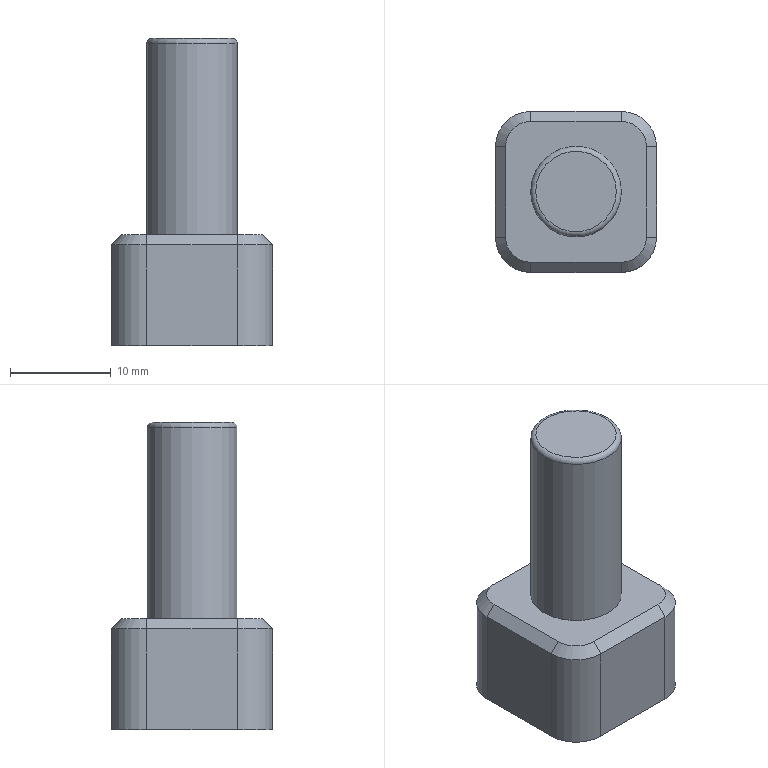NC program | NX | posted with a generic post | part box 16 x 16 x 30.5 mm
Whole program:
N10 G17 G21 G94 G90
(DYNAMIC_ROUGH , TOOL : D12-36-D12-75-3T_ROUGH)
N12 T01 M6
N14 G53
N16 G17 G0 G90 X-22.031 Y-0.836 S6500 M3
N18 G43 Z51. H1
N20 Z-31.5
N22 G94 G1 X-22.006 Z-31.656 F3000.
N24 X-21.981 Z-31.718
N26 X-21.956 Z-31.763
N28 X-21.931 Y-0.835 Z-31.8
N30 X-21.906 Z-31.831
N32 X-21.881 Z-31.857
N34 X-21.856 Y-0.834 Z-31.88
N36 X-21.831 Z-31.9
N38 X-21.806 Z-31.918
N40 X-21.781 Y-0.833 Z-31.933
N42 X-21.756 Z-31.947
N44 X-21.731 Z-31.958
N46 X-21.706 Z-31.968
N48 X-21.681 Y-0.832 Z-31.977
N50 X-21.656 Z-31.984
N52 X-21.631 Z-31.99
N54 X-21.606 Y-0.831 Z-31.994
N56 X-21.581 Z-31.997
N58 X-21.556 Z-31.999
N60 X-21.531 Y-0.83 Z-32.
N62 X-19.634 Y-0.808
N64 G3 X-18.514 Y-0.022 R1.212
N66 X-17.509 Y3.609 R109.508
N68 G2 X-12.877 Y12.031 R20.094
N70 X-4.609 Y-16.993 R-17.608
N72 X-17.194 Y-3.694 R17.471
N74 X-16.874 Y2.692 R16.424
N76 X-10.325 Y13.171 R18.361
N78 X0.613 Y-16.701 R-16.719
N80 X-15.618 Y-5.888 R16.611
N82 X-15.923 Y2.853 R15.623
N84 X-12.605 Y9.692 R17.498
N86 G1 X-12.372 Y10.081
N88 X-11.422 Y11.223
N90 G2 X4.265 Y15.209 R16.422
N92 X8.789 Y13.136 R16.46
N94 G1 X10.173 Y12.306
N96 X11.324 Y11.323
N98 G2 X15.746 Y-1.31 R16.696
N100 X13.113 Y-8.829 R16.055
N102 G1 X12.465 Y-9.948
N104 X11.561 Y-11.077
N106 G2 X6.151 Y-14.604 R15.975
N108 X-8.666 Y-13.208 R15.981
N110 G1 X-9.956 Y-12.46
N112 X-11.085 Y-11.554
N114 G2 X-15.107 Y2.306 R15.032
N116 X-14.081 Y5.563 R21.458
N118 G1 X-14.035 Y5.983
N120 X-13.695 Y7.429
N122 X-13.136 Y8.806
N124 X-12.372 Y10.081
N126 X-11.422 Y11.223
N128 X-10.308 Y12.206
N130 X-9.056 Y13.007
N132 X-7.696 Y13.605
N134 G2 X-4.061 Y14.572 R59.469
N136 X4.693 Y14.136 R17.004
N138 G1 X6.011 Y14.031
N140 X7.483 Y13.677
N142 X8.813 Y13.126
N144 X7.483 Y13.677
N146 X6.011 Y14.031
N148 G2 X1.513 Y14.441 R319.051
N150 G3 X-3.781 Y14.15 R19.844
N152 X-7.217 Y13.733 R9.939
N154 G2 X-4.48 Y14.149 R9.046
N156 G1 X4.501 Y14.15
N158 X6.011 Y14.031
N160 X7.483 Y13.677
N162 X8.882 Y13.098
N164 X10.173 Y12.306
N166 X11.324 Y11.323
N168 X12.308 Y10.171
N170 X13.099 Y8.88
N172 G2 X14.216 Y5.603 R17.673
N174 X14.691 Y-2.504 R18.171
N176 X14.133 Y-4.728 R33.317
N178 X13.099 Y-8.853 R9.647
N180 G3 X14.133 Y-4.728 R9.657
N182 X14.475 Y-0.898 R93.828
N184 X14.15 Y3.737 R22.162
N186 X14.031 Y6.008 R16.89
N188 G1 X13.678 Y7.481
N190 X14.031 Y6.008
N192 G2 X14.15 Y3.737 R16.89
N194 G1 Y-4.501
N196 X14.041 Y-5.943
N198 X13.719 Y-7.352
N200 X13.189 Y-8.697
N202 X12.465 Y-9.948
N204 X11.561 Y-11.077
N206 X10.5 Y-12.058
N208 X9.303 Y-12.87
N210 X7.999 Y-13.493
N212 G2 X2.893 Y-14.775 R32.888
N214 X-4.707 Y-14.136 R17.035
N216 G1 X-5.945 Y-14.041
N218 X-7.356 Y-13.718
N220 X-8.742 Y-13.164
N222 X-7.356 Y-13.718
N224 X-5.945 Y-14.041
N226 G2 X-1.599 Y-14.437 R199.126
N228 G3 X3.69 Y-14.15 R21.622
N230 X6.616 Y-13.915 R13.138
N232 G2 X3.69 Y-14.15 R13.139
N234 G1 X-4.501
N236 X-5.945 Y-14.041
N238 X-7.356 Y-13.718
N240 X-8.703 Y-13.186
N242 X-9.956 Y-12.46
N244 X-11.085 Y-11.554
N246 X-12.066 Y-10.489
N248 X-12.877 Y-9.29
N250 X-13.5 Y-7.982
N252 G2 X-14.527 Y0.316 R20.12
N254 X-14.15 Y2.618 R39.485
N256 X-14.056 Y5.712 R25.322
N258 G3 X-14.15 Y2.618 R25.322
N260 X-14.201 Y-1.155 R178.517
N262 G2 X-14.143 Y-4.832 R57.727
N264 G3 X-13.919 Y-6.596 R17.533
N266 G2 X-14.15 Y-4.5 R13.212
N268 G1 Y2.015
N270 G3 X-15.409 Y3.226 R1.212
N272 G1 X-17.123 Y3.16
N274 X-17.148 Y3.159 Z-31.999
N276 X-17.173 Y3.158 Z-31.997
N278 X-17.198 Y3.157 Z-31.994
N280 X-17.223 Y3.156 Z-31.99
N282 X-17.248 Y3.155 Z-31.984
N284 X-17.273 Y3.154 Z-31.977
N286 X-17.298 Z-31.968
N288 X-17.323 Y3.153 Z-31.958
N290 X-17.348 Y3.152 Z-31.947
N292 X-17.373 Y3.151 Z-31.933
N294 X-17.398 Y3.15 Z-31.918
N296 X-17.423 Y3.149 Z-31.9
N298 X-17.448 Y3.148 Z-31.88
N300 X-17.473 Y3.147 Z-31.857
N302 X-17.498 Y3.146 Z-31.831
N304 X-17.523 Y3.145 Z-31.8
N306 X-17.548 Y3.144 Z-31.763
N308 X-17.573 Y3.143 Z-31.718
N310 X-17.598 Y3.142 Z-31.656
N312 X-17.623 Y3.141 Z-31.5
N314 G0 Z51.
N316 X-17.696 Y-0.817
N318 Z-19.5
N320 G1 X-17.671 Z-19.656
N322 X-17.646 Y-0.816 Z-19.718
N324 X-17.621 Y-0.815 Z-19.763
N326 X-17.596 Z-19.8
N328 X-17.571 Y-0.814 Z-19.831
N330 X-17.546 Z-19.857
N332 X-17.521 Y-0.813 Z-19.88
N334 X-17.496 Z-19.9
N336 X-17.471 Y-0.812 Z-19.918
N338 X-17.446 Y-0.811 Z-19.933
N340 X-17.421 Z-19.947
N342 X-17.396 Y-0.81 Z-19.958
N344 X-17.371 Z-19.968
N346 X-17.346 Y-0.809 Z-19.977
N348 X-17.321 Z-19.984
N350 X-17.296 Y-0.808 Z-19.99
N352 X-17.271 Z-19.994
N354 X-17.246 Y-0.807 Z-19.997
N356 X-17.221 Y-0.806 Z-19.999
N358 X-17.196 Z-20.
N360 X-15.279 Y-0.762
N362 G3 X-14.179 Y0.003 R1.212
N364 X-13.762 Y2.301 R9.377
N366 X-13.691 Y4.496 R14.389
N368 G1 X-13.579 Y5.935
N370 X-13.242 Y7.339
N372 X-12.69 Y8.672
N374 X-11.936 Y9.903
N376 X-10.998 Y11.
N378 X-9.901 Y11.937
N380 X-8.67 Y12.691
N382 X-7.336 Y13.243
N384 X-5.933 Y13.579
N386 X-4.495 Y13.691
N388 X4.496
N390 X5.935 Y13.579
N392 X7.339 Y13.242
N394 X8.672 Y12.69
N396 X9.903 Y11.936
N398 X11. Y10.998
N400 X11.937 Y9.901
N402 X12.691 Y8.67
N404 X13.243 Y7.336
N406 X13.579 Y5.933
N408 X13.691 Y4.495
N410 Y-4.496
N412 X13.579 Y-5.935
N414 X13.242 Y-7.339
N416 X12.69 Y-8.672
N418 X11.936 Y-9.903
N420 X10.998 Y-11.
N422 X9.901 Y-11.937
N424 X8.67 Y-12.691
N426 X7.336 Y-13.243
N428 X5.933 Y-13.579
N430 X4.495 Y-13.691
N432 X-4.496
N434 X-5.935 Y-13.579
N436 X-7.339 Y-13.242
N438 X-8.672 Y-12.69
N440 X-9.903 Y-11.936
N442 X-11. Y-10.998
N444 X-11.937 Y-9.901
N446 X-12.691 Y-8.67
N448 X-13.243 Y-7.336
N450 X-13.579 Y-5.933
N452 X-13.691 Y-4.495
N454 Y3.155
N456 G3 X-14.83 Y4.365 R1.212
N458 G1 X-16.665 Y4.477
N460 X-16.69 Y4.479 Z-19.999
N462 X-16.715 Y4.48 Z-19.997
N464 X-16.74 Y4.482 Z-19.994
N466 X-16.765 Y4.483 Z-19.99
N468 X-16.79 Y4.485 Z-19.984
N470 X-16.815 Y4.486 Z-19.977
N472 X-16.84 Y4.488 Z-19.968
N474 X-16.864 Y4.489 Z-19.958
N476 X-16.889 Y4.491 Z-19.947
N478 X-16.914 Y4.492 Z-19.933
N480 X-16.939 Y4.494 Z-19.918
N482 X-16.964 Y4.495 Z-19.9
N484 X-16.989 Y4.497 Z-19.88
N486 X-17.014 Y4.498 Z-19.857
N488 X-17.039 Y4.5 Z-19.831
N490 X-17.064 Y4.501 Z-19.8
N492 X-17.089 Y4.503 Z-19.763
N494 X-17.114 Y4.504 Z-19.718
N496 X-17.139 Y4.506 Z-19.656
N498 X-17.164 Y4.508 Z-19.5
N500 G0 Z51.
N502 X-17.237 Y-0.777
N504 Z-19.
N506 G1 X-17.212 Y-0.778 Z-19.156
N508 X-17.187 Y-0.779 Z-19.218
N510 X-17.162 Y-0.78 Z-19.263
N512 X-17.137 Y-0.781 Z-19.3
N514 X-17.112 Y-0.782 Z-19.331
N516 X-17.087 Y-0.783 Z-19.357
N518 X-17.062 Y-0.784 Z-19.38
N520 X-17.037 Y-0.785 Z-19.4
N522 X-17.013 Y-0.786 Z-19.418
N524 X-16.988 Y-0.787 Z-19.433
N526 X-16.963 Y-0.788 Z-19.447
N528 X-16.938 Y-0.789 Z-19.458
N530 X-16.913 Y-0.79 Z-19.468
N532 X-16.888 Y-0.791 Z-19.477
N534 X-16.863 Y-0.792 Z-19.484
N536 X-16.838 Y-0.793 Z-19.49
N538 X-16.813 Y-0.794 Z-19.494
N540 X-16.788 Y-0.795 Z-19.497
N542 X-16.763 Y-0.796 Z-19.499
N544 X-16.738 Y-0.797 Z-19.5
N546 X-14.936 Y-0.87
N548 G3 X-13.721 Y0.011 R1.212
N550 X-13.27 Y2.769 R13.146
N552 X-13.191 Y4.502 R10.466
N554 G1 X-13.084 Y5.862
N556 X-12.765 Y7.188
N558 X-12.243 Y8.448
N560 X-11.53 Y9.611
N562 X-10.644 Y10.648
N564 X-9.606 Y11.533
N566 X-8.443 Y12.245
N568 X-7.183 Y12.767
N570 X-5.857 Y13.085
N572 X-4.498 Y13.191
N574 X4.502
N576 X5.862 Y13.084
N578 X7.188 Y12.765
N580 X8.448 Y12.243
N582 X9.611 Y11.53
N584 X10.648 Y10.644
N586 X11.533 Y9.606
N588 X12.245 Y8.443
N590 X12.767 Y7.183
N592 X13.085 Y5.857
N594 X13.191 Y4.498
N596 Y-4.502
N598 X13.084 Y-5.862
N600 X12.765 Y-7.188
N602 X12.243 Y-8.448
N604 X11.53 Y-9.611
N606 X10.644 Y-10.648
N608 X9.606 Y-11.533
N610 X8.443 Y-12.245
N612 X7.183 Y-12.767
N614 X5.857 Y-13.085
N616 X4.498 Y-13.191
N618 X-4.499
N620 X-5.859 Y-13.084
N622 X-7.186 Y-12.766
N624 X-8.446 Y-12.244
N626 X-9.609 Y-11.531
N628 X-10.647 Y-10.645
N630 X-11.532 Y-9.607
N632 X-12.245 Y-8.444
N634 X-12.767 Y-7.184
N636 X-13.085 Y-5.857
N638 X-13.191 Y-4.498
N640 Y3.602
N642 G3 X-14.264 Y4.806 R1.212
N644 G1 X-16.133 Y5.022
N646 X-16.158 Y5.025 Z-19.499
N648 X-16.183 Y5.028 Z-19.497
N650 X-16.208 Y5.031 Z-19.494
N652 X-16.232 Y5.034 Z-19.49
N654 X-16.257 Y5.036 Z-19.484
N656 X-16.282 Y5.039 Z-19.477
N658 X-16.307 Y5.042 Z-19.468
N660 X-16.332 Y5.045 Z-19.458
N662 X-16.357 Y5.048 Z-19.447
N664 X-16.381 Y5.051 Z-19.433
N666 X-16.406 Y5.054 Z-19.418
N668 X-16.431 Y5.057 Z-19.4
N670 X-16.456 Y5.059 Z-19.38
N672 X-16.481 Y5.062 Z-19.357
N674 X-16.506 Y5.065 Z-19.331
N676 X-16.53 Y5.068 Z-19.3
N678 X-16.555 Y5.071 Z-19.263
N680 X-16.58 Y5.074 Z-19.218
N682 X-16.605 Y5.077 Z-19.156
N684 X-16.63 Y5.079 Z-19.
N686 G0 Z51.
N688 X-16.736 Y-1.002
N690 Z-18.5
N692 G1 X-16.711 Y-1.003 Z-18.656
N694 X-16.686 Y-1.004 Z-18.718
N696 X-16.662 Y-1.006 Z-18.763
N698 X-16.637 Y-1.007 Z-18.8
N700 X-16.612 Y-1.008 Z-18.831
N702 X-16.587 Y-1.009 Z-18.857
N704 X-16.562 Y-1.01 Z-18.88
N706 X-16.537 Y-1.011 Z-18.9
N708 X-16.512 Y-1.012 Z-18.918
N710 X-16.487 Y-1.014 Z-18.933
N712 X-16.462 Y-1.015 Z-18.947
N714 X-16.437 Y-1.016 Z-18.958
N716 X-16.412 Y-1.017 Z-18.968
N718 X-16.387 Y-1.018 Z-18.977
N720 X-16.362 Y-1.019 Z-18.984
N722 X-16.337 Y-1.02 Z-18.99
N724 X-16.312 Y-1.021 Z-18.994
N726 X-16.287 Y-1.023 Z-18.997
N728 X-16.262 Y-1.024 Z-18.999
N730 X-16.237 Y-1.025 Z-19.
N732 X-14.444 Y-1.106
N734 G3 X-13.22 Y-0.217 R1.212
N736 X-12.733 Y2.997 R15.221
N738 G2 X-11.104 Y7.989 R10.286
N740 X-6.47 Y11.405 R9.167
N742 X-1.131 Y12.391 R20.302
N744 X3.634 Y12.48 R34.532
N746 X9.706 Y9.446 R8.673
N748 X11.926 Y4.519 R11.385
N750 X12.505 Y-1.25 R33.126
N752 X12.171 Y-5.404 R13.639
N754 X7.066 Y-11.135 R8.553
N756 X1.731 Y-12.334 R17.609
N758 X-3.572 Y-12.484 R36.466
N760 X-9.622 Y-9.545 R8.708
N762 X-11.867 Y-4.784 R11.079
N764 X-12.225 Y-0.176 R18.232
N766 X-11.67 Y4.184 R15.813
N768 X-6.805 Y9.843 R9.659
N770 X-1.005 Y11.544 R17.14
N772 X3.563 Y11.522 R13.748
N774 X9.515 Y7.172 R9.137
N776 X11.431 Y1.589 R15.411
N778 X11.586 Y-3.159 R15.186
N780 X7.329 Y-9.414 R9.056
N782 X1.813 Y-11.393 R14.998
N784 X-3.023 Y-11.606 R15.829
N786 X-9.555 Y-7.087 R9.041
N788 X-11.281 Y-0.946 R13.939
N790 X-9.327 Y6.004 R10.123
N792 X-4.895 Y9.435 R11.414
N794 G1 X-4.557 Y9.626
N796 G2 X-2.405 Y10.373 R13.698
N798 X2.893 Y10.456 R10.746
N800 X8.032 Y6.95 R9.543
N802 G1 X8.552 Y6.347
N804 X9.386 Y5.032
N806 G2 X10.103 Y3.354 R19.792
N808 X10.71 Y-1.419 R12.715
N810 X7.253 Y-7.799 R9.425
N812 G1 X6.05 Y-8.765
N814 X4.721 Y-9.547
N816 G2 X2.903 Y-10.241 R15.388
N818 X-2.083 Y-10.622 R11.78
N820 X-7.566 Y-7.458 R9.091
N822 G1 X-7.968 Y-7.066
N824 X-8.905 Y-5.841
N826 X-9.644 Y-4.518
N828 X-10.188 Y-3.103
N830 X-10.525 Y-1.625
N832 X-10.649 Y-0.116
N834 X-10.558 Y1.398
N836 X-10.252 Y2.883
N838 X-9.739 Y4.309
N840 X-9.029 Y5.648
N842 X-8.136 Y6.872
N844 X-7.078 Y7.957
N846 X-5.877 Y8.882
N848 X-4.557 Y9.626
N850 X-3.144 Y10.175
N852 X-1.668 Y10.518
N854 G2 X2.336 Y10.391 R11.489
N856 G1 X3.625 Y10.014
N858 X5.046 Y9.379
N860 X6.359 Y8.543
N862 X7.536 Y7.525
N864 X8.552 Y6.347
N866 X9.386 Y5.032
N868 X10.019 Y3.611
N870 X10.438 Y2.112
N872 X10.635 Y0.568
N874 X10.604 Y-0.988
N876 X10.347 Y-2.523
N878 X9.868 Y-4.004
N880 X9.179 Y-5.4
N882 X8.303 Y-6.669
N884 X7.253 Y-7.799
N886 X6.05 Y-8.765
N888 X4.721 Y-9.547
N890 X3.292 Y-10.128
N892 X1.795 Y-10.498
N894 X0.26 Y-10.647
N896 X-1.281 Y-10.573
N898 X-2.795 Y-10.277
N900 X-4.25 Y-9.765
N902 X-5.616 Y-9.049
N904 X-6.864 Y-8.143
N906 X-7.573 Y-7.452
N908 G3 X-9.006 Y-7.259 R1.212
N910 G1 X-10.803 Y-8.254
N912 X-10.825 Y-8.266 Z-18.999
N914 X-10.847 Y-8.279 Z-18.997
N916 X-10.869 Y-8.291 Z-18.994
N918 X-10.89 Y-8.303 Z-18.99
N920 X-10.912 Y-8.315 Z-18.984
N922 X-10.934 Y-8.327 Z-18.977
N924 X-10.956 Y-8.339 Z-18.968
N926 X-10.978 Y-8.351 Z-18.958
N928 X-11. Y-8.363 Z-18.947
N930 X-11.022 Y-8.375 Z-18.933
N932 X-11.043 Y-8.388 Z-18.918
N934 X-11.065 Y-8.4 Z-18.9
N936 X-11.087 Y-8.412 Z-18.88
N938 X-11.109 Y-8.424 Z-18.857
N940 X-11.131 Y-8.436 Z-18.831
N942 X-11.153 Y-8.448 Z-18.8
N944 X-11.175 Y-8.46 Z-18.763
N946 X-11.197 Y-8.472 Z-18.718
N948 X-11.218 Y-8.484 Z-18.656
N950 X-11.24 Y-8.497 Z-18.5
N952 G0 Z51.
N954 X-14.192 Y-1.19
N956 Z0.5
N958 G1 X-14.167 Z0.344
N960 X-14.142 Y-1.191 Z0.282
N962 X-14.117 Z0.237
N964 X-14.092 Z0.2
N966 X-14.067 Y-1.192 Z0.169
N968 X-14.042 Z0.143
N970 X-14.017 Z0.12
N972 X-13.992 Y-1.193 Z0.1
N974 X-13.967 Z0.082
N976 X-13.942 Z0.067
N978 X-13.917 Y-1.194 Z0.053
N980 X-13.892 Z0.042
N982 X-13.867 Z0.032
N984 X-13.842 Y-1.195 Z0.023
N986 X-13.817 Z0.016
N988 X-13.792 Z0.01
N990 X-13.767 Y-1.196 Z0.006
N992 X-13.742 Z0.003
N994 X-13.717 Z0.001
N996 X-13.692 Y-1.197 Z0.
N998 X-11.843 Y-1.222
N1000 G3 X-10.676 Y-0.388 R1.212
N1002 G1 X-10.328 Y0.855
N1004 X-10.308 Y1.235
N1006 X-10.026 Y2.695
N1008 X-9.538 Y4.099
N1010 X-8.854 Y5.42
N1012 X-7.989 Y6.629
N1014 X-6.96 Y7.703
N1016 X-5.788 Y8.618
N1018 X-4.498 Y9.357
N1020 X-3.115 Y9.903
N1022 X-1.668 Y10.247
N1024 X-0.193 Y10.38
N1026 X1.285 Y10.302
N1028 X2.737 Y10.014
N1030 X4.168 Y9.508
N1032 X5.509 Y8.799
N1034 X6.733 Y7.902
N1036 X7.813 Y6.836
N1038 X8.726 Y5.624
N1040 X9.453 Y4.292
N1042 X9.977 Y2.869
N1044 X10.289 Y1.384
N1046 X10.381 Y-0.131
N1048 X10.251 Y-1.643
N1050 X9.902 Y-3.119
N1052 X9.341 Y-4.529
N1054 X8.581 Y-5.843
N1056 X7.614 Y-7.057
N1058 X6.476 Y-8.114
N1060 X5.193 Y-8.989
N1062 X3.795 Y-9.663
N1064 X2.311 Y-10.121
N1066 X0.775 Y-10.353
N1068 X-0.778 Y-10.352
N1070 X-2.313 Y-10.121
N1072 X-3.797 Y-9.662
N1074 X-5.195 Y-8.988
N1076 X-6.478 Y-8.113
N1078 X-7.615 Y-7.056
N1080 X-8.583 Y-5.841
N1082 X-9.329 Y-4.555
N1084 X-9.884 Y-3.175
N1086 X-10.236 Y-1.731
N1088 X-10.379 Y-0.252
N1090 X-10.323 Y0.917
N1092 G3 X-11.096 Y2.105 R1.212
N1094 G1 X-13.024 Y2.851
N1096 X-13.047 Y2.86 Z0.001
N1098 X-13.071 Y2.869 Z0.003
N1100 X-13.094 Y2.878 Z0.006
N1102 X-13.117 Y2.887 Z0.01
N1104 X-13.141 Y2.896 Z0.016
N1106 X-13.164 Y2.905 Z0.023
N1108 X-13.187 Y2.914 Z0.032
N1110 X-13.211 Y2.923 Z0.042
N1112 X-13.234 Y2.932 Z0.053
N1114 X-13.257 Y2.941 Z0.067
N1116 X-13.281 Y2.95 Z0.082
N1118 X-13.304 Y2.959 Z0.1
N1120 X-13.327 Y2.968 Z0.12
N1122 X-13.351 Y2.977 Z0.143
N1124 X-13.374 Y2.986 Z0.169
N1126 X-13.397 Y2.995 Z0.2
N1128 X-13.421 Y3.004 Z0.237
N1130 X-13.444 Y3.013 Z0.282
N1132 X-13.467 Y3.022 Z0.344
N1134 X-13.49 Y3.031 Z0.5
N1136 G0 Z51.
N1138 X-13.917 Y-0.784
N1140 Z0.6
N1142 G1 X-13.892 Y-0.785 Z0.444
N1144 X-13.867 Z0.382
N1146 X-13.842 Z0.337
N1148 X-13.817 Y-0.786 Z0.3
N1150 X-13.792 Z0.269
N1152 X-13.767 Y-0.787 Z0.243
N1154 X-13.742 Z0.22
N1156 X-13.717 Z0.2
N1158 X-13.692 Y-0.788 Z0.182
N1160 X-13.667 Z0.167
N1162 X-13.642 Z0.153
N1164 X-13.617 Y-0.789 Z0.142
N1166 X-13.592 Z0.132
N1168 X-13.567 Y-0.79 Z0.123
N1170 X-13.542 Z0.116
N1172 X-13.517 Z0.11
N1174 X-13.492 Y-0.791 Z0.106
N1176 X-13.467 Z0.103
N1178 X-13.442 Y-0.792 Z0.101
N1180 X-13.417 Z0.1
N1182 X-11.572 Y-0.821
N1184 G3 X-10.4 Y0.016 R1.212
N1186 G2 X-8.051 Y4.936 R16.238
N1188 X0.414 Y9.016 R9.817
N1190 X5.354 Y-7.138 R8.995
N1192 X-6.951 Y-5.556 R8.863
N1194 X-7.773 Y2.288 R8.102
N1196 X0.46 Y7.324 R8.025
N1198 X6.679 Y-2.009 R7.245
N1200 X-0.445 Y-6.826 R6.85
N1202 X-5.618 Y-0.645 R5.75
N1204 X-4.558 Y1.999 R5.63
N1206 G1 X-4.405 Y2.221
N1208 X-4.391 Y2.242 Z0.101
N1210 X-4.377 Y2.263 Z0.103
N1212 X-4.363 Y2.283 Z0.106
N1214 X-4.348 Y2.304 Z0.11
N1216 X-4.334 Y2.324 Z0.116
N1218 X-4.32 Y2.345 Z0.123
N1220 X-4.306 Y2.366 Z0.132
N1222 X-4.292 Y2.386 Z0.142
N1224 X-4.278 Y2.407 Z0.153
N1226 X-4.263 Y2.427 Z0.167
N1228 X-4.249 Y2.448 Z0.182
N1230 X-4.235 Y2.469 Z0.2
N1232 X-4.221 Y2.489 Z0.22
N1234 X-4.207 Y2.51 Z0.243
N1236 X-4.193 Y2.53 Z0.269
N1238 X-4.179 Y2.551 Z0.3
N1240 X-4.164 Y2.572 Z0.337
N1242 X-4.15 Y2.592 Z0.382
N1244 X-4.136 Y2.613 Z0.444
N1246 X-4.122 Y2.633 Z0.6
N1248 G0 Z51.
N1250 M5
(FLOOR_WALL , TOOL : D12-36-D12-120-3T_FINISH)
N1252 T02 M6
N1254 G53
N1256 G17 G0 G90 X-12.962 Y0.999 S6500 M3
N1258 G43 Z53. H2
N1260 Z3.
N1262 G94 G1 Z0. F300.
N1264 X-9.95
N1266 X9.95 Y1.
N1268 X12.961
N1270 Z3.
N1272 G0 Z53.
(PLANAR_MILL_COPY , TOOL : D12-36-D12-120-3T_FINISH)
N1274 X12.699 Y1.965
N1276 Z50.
N1278 Z-17.5
N1280 G1 Z-19.5
N1282 G41 X12.502 Y2. D2
N1284 G3 X10.502 Y0. R2.
N1286 G2 X0. Y-10.502 R10.502
N1288 X10.502 Y0. R-10.502
N1290 G3 X12.502 Y-2. R2.
N1292 G40
N1294 G1 X12.699 Y-1.965
N1296 X12.698 Y1.965
N1298 G41 X12.501 Y2.
N1300 G3 X10.501 Y0. R2.
N1302 G2 X0. Y-10.501 R10.501
N1304 X10.501 Y0. R-10.501
N1306 G3 X12.501 Y-2. R2.
N1308 G40
N1310 G1 X12.698 Y-1.965
N1312 X12.697 Y1.965
N1314 G41 X12.5 Y2.
N1316 G3 X10.5 Y0. R2.
N1318 G2 X0. Y-10.5 R10.5
N1320 X10.5 Y0. R-10.5
N1322 G3 X12.5 Y-2. R2.
N1324 G40
N1326 G1 X12.697 Y-1.965
N1328 Z-17.5
N1330 G0 Z50.
(PLANAR_MILL , TOOL : D12-36-D12-120-3T_FINISH)
N1332 X-16.197 Y-6.465
N1334 Z-29.
N1336 G1 Z-31.
N1338 G41 X-16. Y-6.5
N1340 G3 X-14. Y-4.5 R2.
N1342 G1 Y4.5
N1344 G2 X-4.5 Y14. R9.5
N1346 G1 X4.5
N1348 G2 X14. Y4.5 R9.5
N1350 G1 Y-4.5
N1352 G2 X4.5 Y-14. R9.5
N1354 G1 X-4.5
N1356 G2 X-14. Y-4.5 R9.5
N1358 G3 X-16. Y-2.5 R2.
N1360 G40
N1362 G1 X-16.197 Y-2.535
N1364 Y-6.465
N1366 G41 X-16. Y-6.5
N1368 G3 X-14. Y-4.5 R2.
N1370 G1 Y4.5
N1372 G2 X-4.5 Y14. R9.5
N1374 G1 X4.5
N1376 G2 X14. Y4.5 R9.5
N1378 G1 Y-4.5
N1380 G2 X4.5 Y-14. R9.5
N1382 G1 X-4.5
N1384 G2 X-14. Y-4.5 R9.5
N1386 G3 X-16. Y-2.5 R2.
N1388 G40
N1390 G1 X-16.197 Y-2.535
N1392 Z-29.
N1394 G0 Z50.
N1396 M5
(PLANAR_MILL_COPY_1 , TOOL : CHAMFER_D8-90DEG)
N1398 T03 M6
N1400 G53
N1402 G17 G0 G90 X-13.685 Y-6.326 S3000 M3
N1404 G43 Z50. H3
N1406 Z-21.
N1408 G94 G1 Z-23. F800.
N1410 G41 X-12.7 Y-6.5 D3
N1412 G3 X-10.7 Y-4.5 R2.
N1414 G1 Y4.5
N1416 G2 X-4.5 Y10.7 R6.2
N1418 G1 X4.5
N1420 G2 X10.7 Y4.5 R6.2
N1422 G1 Y-4.5
N1424 G2 X4.5 Y-10.7 R6.2
N1426 G1 X-4.5
N1428 G2 X-10.7 Y-4.5 R6.2
N1430 G3 X-12.7 Y-2.5 R2.
N1432 G40
N1434 G1 X-13.685 Y-2.674
N1436 Z-21.
N1438 G0 Z50.
N1440 M5
(ZLEVEL_PROFILE_STEEP , TOOL : MILL)
N1442 T04 M6
N1444 G53
N1446 G17 G0 G90 X-9.646 Y-1.8 S4500 M3
N1448 G43 Z51. H4
N1450 Z0.95
N1452 G94 G1 Z-0.05 F2000.
N1454 X-8.612
N1456 G3 X-6.812 Y0. R1.8
N1458 G2 X0. Y6.812 R6.812
N1460 X-6.812 Y0. R-6.812
N1462 G1 X-6.936 Z-0.1
N1464 G2 X0. Y6.936 R6.936
N1466 X-6.936 Y0. R-6.936
N1468 G1 X-7.027 Z-0.15
N1470 G2 X0. Y7.027 R7.027
N1472 X-7.027 Y0. R-7.027
N1474 G1 X-7.1 Z-0.2
N1476 G2 X0. Y7.1 R7.1
N1478 X-7.1 Y0. R-7.1
N1480 G1 X-7.161 Z-0.25
N1482 G2 X0. Y7.161 R7.161
N1484 X-7.161 Y0. R-7.161
N1486 G1 X-7.214 Z-0.3
N1488 G2 X0. Y7.214 R7.214
N1490 X-7.214 Y0. R-7.214
N1492 G1 X-7.26 Z-0.35
N1494 G2 X0. Y7.26 R7.26
N1496 X-7.26 Y0. R-7.26
N1498 G1 X-7.3 Z-0.4
N1500 G2 X0. Y7.3 R7.3
N1502 X-7.3 Y0. R-7.3
N1504 G1 X-7.335 Z-0.45
N1506 G2 X0. Y7.335 R7.335
N1508 X-7.335 Y0. R-7.335
N1510 G1 X-7.366 Z-0.5
N1512 G2 X0. Y7.366 R7.366
N1514 X-7.366 Y0. R-7.366
N1516 G1 X-7.393 Z-0.55
N1518 G2 X0. Y7.393 R7.393
N1520 X-7.393 Y0. R-7.393
N1522 G1 X-7.417 Z-0.6
N1524 G2 X0. Y7.417 R7.417
N1526 X-7.417 Y0. R-7.417
N1528 G1 X-7.437 Z-0.65
N1530 G2 X0. Y7.437 R7.437
N1532 X-7.437 Y0. R-7.437
N1534 G1 X-7.454 Z-0.7
N1536 G2 X0. Y7.454 R7.454
N1538 X-7.454 Y0. R-7.454
N1540 G1 X-7.468 Z-0.75
N1542 G2 X0. Y7.468 R7.468
N1544 X-7.468 Y0. R-7.468
N1546 G1 X-7.48 Z-0.8
N1548 G2 X0. Y7.48 R7.48
N1550 X-7.48 Y0. R-7.48
N1552 G1 X-7.489 Z-0.85
N1554 G2 X0. Y7.489 R7.489
N1556 X-7.489 Y0. R-7.489
N1558 G1 X-7.495 Z-0.9
N1560 G2 X0. Y7.495 R7.495
N1562 X-7.495 Y0. R-7.495
N1564 G1 X-7.499 Z-0.95
N1566 G2 X0. Y7.499 R7.499
N1568 X-7.499 Y0. R-7.499
N1570 G1 X-7.5 Z-1.
N1572 G2 X-7.441 Y0.942 R7.5
N1574 G1 X-7.351 Y1.488
N1576 G2 X6.425 Y3.869 R7.5
N1578 G1 X6.748 Y3.274
N1580 G2 X-7.5 Y0. R-7.5
N1582 G3 X-9.3 Y1.8 R1.8
N1584 G1 X-10.34
N1586 Z0.
N1588 G0 Z51.
N1590 M5
N1592 M2